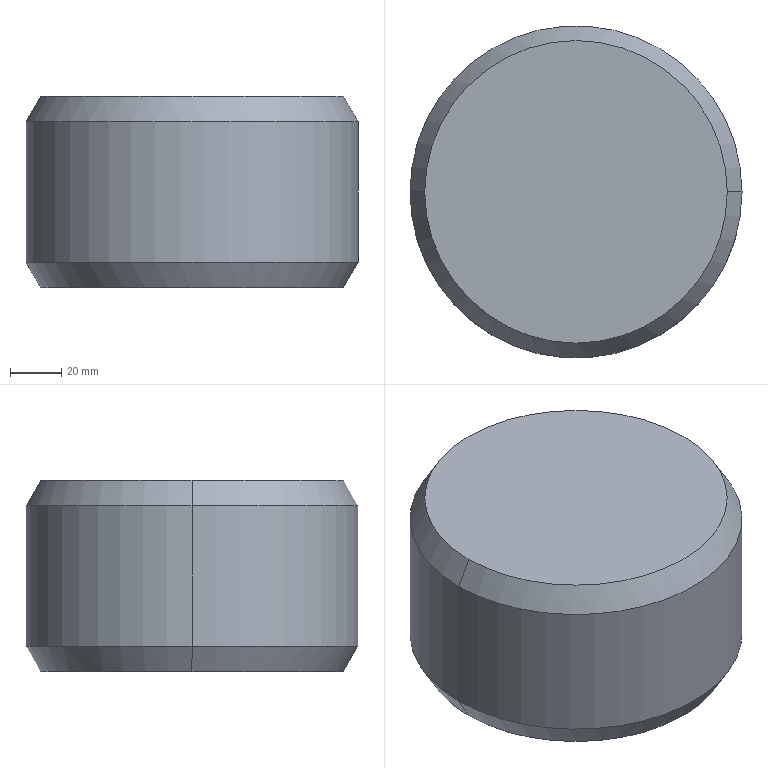Part | SolidWorks | features Chamfer 1, Extrusion 1 | 1 solid | 8 faces | box 130 x 130 x 75 mm | volume 972611 mm3 | cone 4 | cylinder 2 | plane 2 | commonest cylinder face diameters 130 x2
STEP:
#1=CARTESIAN_POINT('',(-59.226,0.,0.));
#2=VERTEX_POINT('',#1);
#3=CARTESIAN_POINT('',(59.226,0.,0.));
#4=VERTEX_POINT('',#3);
#5=CARTESIAN_POINT('',(0.,0.,0.));
#6=DIRECTION('',(0.,0.,-1.));
#7=DIRECTION('',(1.,0.,0.));
#8=AXIS2_PLACEMENT_3D('',#5,#6,#7);
#9=CIRCLE('',#8,59.226);
#10=EDGE_CURVE('',#2,#4,#9,.T.);
#11=ORIENTED_EDGE('',*,*,#10,.F.);
#12=CARTESIAN_POINT('',(-65.,0.,10.));
#13=VERTEX_POINT('',#12);
#14=CARTESIAN_POINT('',(-65.,0.,10.));
#15=DIRECTION('',(-0.5,0.,0.866));
#16=VECTOR('',#15,1000.);
#17=LINE('',#14,#16);
#18=EDGE_CURVE('',#2,#13,#17,.T.);
#19=ORIENTED_EDGE('',*,*,#18,.T.);
#20=CARTESIAN_POINT('',(65.,0.,10.));
#21=VERTEX_POINT('',#20);
#22=CARTESIAN_POINT('',(0.,0.,10.));
#23=DIRECTION('',(0.,0.,1.));
#24=DIRECTION('',(1.,0.,0.));
#25=AXIS2_PLACEMENT_3D('',#22,#23,#24);
#26=CIRCLE('',#25,65.);
#27=EDGE_CURVE('',#21,#13,#26,.T.);
#28=ORIENTED_EDGE('',*,*,#27,.F.);
#29=CARTESIAN_POINT('',(65.,0.,10.));
#30=DIRECTION('',(0.5,0.,0.866));
#31=VECTOR('',#30,1000.);
#32=LINE('',#29,#31);
#33=EDGE_CURVE('',#4,#21,#32,.T.);
#34=ORIENTED_EDGE('',*,*,#33,.F.);
#35=EDGE_LOOP('',(#11,#19,#28,#34));
#36=FACE_OUTER_BOUND('',#35,.T.);
#37=CARTESIAN_POINT('',(0.,0.,10.));
#38=DIRECTION('',(0.,0.,1.));
#39=DIRECTION('',(1.,0.,0.));
#40=AXIS2_PLACEMENT_3D('',#37,#38,#39);
#41=CONICAL_SURFACE('',#40,65.,0.5236);
#42=ADVANCED_FACE('',(#36),#41,.T.);
#43=CARTESIAN_POINT('',(59.226,0.,75.));
#44=VERTEX_POINT('',#43);
#45=CARTESIAN_POINT('',(-59.226,0.,75.));
#46=VERTEX_POINT('',#45);
#47=CARTESIAN_POINT('',(0.,0.,75.));
#48=DIRECTION('',(0.,0.,1.));
#49=DIRECTION('',(1.,0.,0.));
#50=AXIS2_PLACEMENT_3D('',#47,#48,#49);
#51=CIRCLE('',#50,59.226);
#52=EDGE_CURVE('',#44,#46,#51,.T.);
#53=ORIENTED_EDGE('',*,*,#52,.F.);
#54=CARTESIAN_POINT('',(65.,0.,65.));
#55=VERTEX_POINT('',#54);
#56=CARTESIAN_POINT('',(59.226,0.,75.));
#57=DIRECTION('',(0.5,0.,-0.866));
#58=VECTOR('',#57,1000.);
#59=LINE('',#56,#58);
#60=EDGE_CURVE('',#44,#55,#59,.T.);
#61=ORIENTED_EDGE('',*,*,#60,.T.);
#62=CARTESIAN_POINT('',(-65.,0.,65.));
#63=VERTEX_POINT('',#62);
#64=CARTESIAN_POINT('',(0.,0.,65.));
#65=DIRECTION('',(0.,0.,-1.));
#66=DIRECTION('',(1.,0.,0.));
#67=AXIS2_PLACEMENT_3D('',#64,#65,#66);
#68=CIRCLE('',#67,65.);
#69=EDGE_CURVE('',#63,#55,#68,.T.);
#70=ORIENTED_EDGE('',*,*,#69,.F.);
#71=CARTESIAN_POINT('',(-59.226,0.,75.));
#72=DIRECTION('',(-0.5,0.,-0.866));
#73=VECTOR('',#72,1000.);
#74=LINE('',#71,#73);
#75=EDGE_CURVE('',#46,#63,#74,.T.);
#76=ORIENTED_EDGE('',*,*,#75,.F.);
#77=EDGE_LOOP('',(#53,#61,#70,#76));
#78=FACE_OUTER_BOUND('',#77,.T.);
#79=CARTESIAN_POINT('',(0.,0.,75.));
#80=DIRECTION('',(0.,0.,-1.));
#81=DIRECTION('',(-1.,0.,0.));
#82=AXIS2_PLACEMENT_3D('',#79,#80,#81);
#83=CONICAL_SURFACE('',#82,59.226,0.5236);
#84=ADVANCED_FACE('',(#78),#83,.T.);
#85=ORIENTED_EDGE('',*,*,#69,.T.);
#86=CARTESIAN_POINT('',(65.,0.,75.));
#87=DIRECTION('',(0.,0.,-1.));
#88=VECTOR('',#87,1000.);
#89=LINE('',#86,#88);
#90=EDGE_CURVE('',#55,#21,#89,.T.);
#91=ORIENTED_EDGE('',*,*,#90,.T.);
#92=ORIENTED_EDGE('',*,*,#27,.T.);
#93=CARTESIAN_POINT('',(-65.,0.,75.));
#94=DIRECTION('',(0.,0.,-1.));
#95=VECTOR('',#94,1000.);
#96=LINE('',#93,#95);
#97=EDGE_CURVE('',#63,#13,#96,.T.);
#98=ORIENTED_EDGE('',*,*,#97,.F.);
#99=EDGE_LOOP('',(#85,#91,#92,#98));
#100=FACE_OUTER_BOUND('',#99,.T.);
#101=CARTESIAN_POINT('',(0.,0.,75.));
#102=DIRECTION('',(0.,0.,-1.));
#103=DIRECTION('',(-1.,0.,0.));
#104=AXIS2_PLACEMENT_3D('',#101,#102,#103);
#105=CYLINDRICAL_SURFACE('',#104,65.);
#106=ADVANCED_FACE('',(#100),#105,.T.);
#107=ORIENTED_EDGE('',*,*,#90,.F.);
#108=CARTESIAN_POINT('',(0.,0.,65.));
#109=DIRECTION('',(0.,0.,-1.));
#110=DIRECTION('',(1.,0.,0.));
#111=AXIS2_PLACEMENT_3D('',#108,#109,#110);
#112=CIRCLE('',#111,65.);
#113=EDGE_CURVE('',#55,#63,#112,.T.);
#114=ORIENTED_EDGE('',*,*,#113,.T.);
#115=ORIENTED_EDGE('',*,*,#97,.T.);
#116=CARTESIAN_POINT('',(0.,0.,10.));
#117=DIRECTION('',(0.,0.,1.));
#118=DIRECTION('',(1.,0.,0.));
#119=AXIS2_PLACEMENT_3D('',#116,#117,#118);
#120=CIRCLE('',#119,65.);
#121=EDGE_CURVE('',#13,#21,#120,.T.);
#122=ORIENTED_EDGE('',*,*,#121,.T.);
#123=EDGE_LOOP('',(#107,#114,#115,#122));
#124=FACE_OUTER_BOUND('',#123,.T.);
#125=CARTESIAN_POINT('',(0.,0.,75.));
#126=DIRECTION('',(0.,0.,-1.));
#127=DIRECTION('',(-1.,0.,0.));
#128=AXIS2_PLACEMENT_3D('',#125,#126,#127);
#129=CYLINDRICAL_SURFACE('',#128,65.);
#130=ADVANCED_FACE('',(#124),#129,.T.);
#131=CARTESIAN_POINT('',(0.,0.,75.));
#132=DIRECTION('',(0.,0.,1.));
#133=DIRECTION('',(1.,0.,0.));
#134=AXIS2_PLACEMENT_3D('',#131,#132,#133);
#135=CIRCLE('',#134,59.226);
#136=EDGE_CURVE('',#46,#44,#135,.T.);
#137=ORIENTED_EDGE('',*,*,#136,.T.);
#138=ORIENTED_EDGE('',*,*,#52,.T.);
#139=EDGE_LOOP('',(#137,#138));
#140=FACE_OUTER_BOUND('',#139,.T.);
#141=CARTESIAN_POINT('',(0.,0.,75.));
#142=DIRECTION('',(0.,0.,1.));
#143=DIRECTION('',(1.,0.,0.));
#144=AXIS2_PLACEMENT_3D('',#141,#142,#143);
#145=PLANE('',#144);
#146=ADVANCED_FACE('',(#140),#145,.T.);
#147=CARTESIAN_POINT('',(0.,0.,0.));
#148=DIRECTION('',(0.,0.,-1.));
#149=DIRECTION('',(1.,0.,0.));
#150=AXIS2_PLACEMENT_3D('',#147,#148,#149);
#151=CIRCLE('',#150,59.226);
#152=EDGE_CURVE('',#4,#2,#151,.T.);
#153=ORIENTED_EDGE('',*,*,#152,.T.);
#154=ORIENTED_EDGE('',*,*,#10,.T.);
#155=EDGE_LOOP('',(#153,#154));
#156=FACE_OUTER_BOUND('',#155,.T.);
#157=CARTESIAN_POINT('',(0.,0.,0.));
#158=DIRECTION('',(0.,0.,1.));
#159=DIRECTION('',(1.,0.,0.));
#160=AXIS2_PLACEMENT_3D('',#157,#158,#159);
#161=PLANE('',#160);
#162=ADVANCED_FACE('',(#156),#161,.F.);
#163=ORIENTED_EDGE('',*,*,#60,.F.);
#164=ORIENTED_EDGE('',*,*,#136,.F.);
#165=ORIENTED_EDGE('',*,*,#75,.T.);
#166=ORIENTED_EDGE('',*,*,#113,.F.);
#167=EDGE_LOOP('',(#163,#164,#165,#166));
#168=FACE_OUTER_BOUND('',#167,.T.);
#169=CARTESIAN_POINT('',(0.,0.,75.));
#170=DIRECTION('',(0.,0.,-1.));
#171=DIRECTION('',(-1.,0.,0.));
#172=AXIS2_PLACEMENT_3D('',#169,#170,#171);
#173=CONICAL_SURFACE('',#172,59.226,0.5236);
#174=ADVANCED_FACE('',(#168),#173,.T.);
#175=ORIENTED_EDGE('',*,*,#18,.F.);
#176=ORIENTED_EDGE('',*,*,#152,.F.);
#177=ORIENTED_EDGE('',*,*,#33,.T.);
#178=ORIENTED_EDGE('',*,*,#121,.F.);
#179=EDGE_LOOP('',(#175,#176,#177,#178));
#180=FACE_OUTER_BOUND('',#179,.T.);
#181=CARTESIAN_POINT('',(0.,0.,10.));
#182=DIRECTION('',(0.,0.,1.));
#183=DIRECTION('',(1.,0.,0.));
#184=AXIS2_PLACEMENT_3D('',#181,#182,#183);
#185=CONICAL_SURFACE('',#184,65.,0.5236);
#186=ADVANCED_FACE('',(#180),#185,.T.);
#187=CLOSED_SHELL('',(#42,#84,#106,#130,#146,#162,#174,#186));
#188=MANIFOLD_SOLID_BREP('',#187);
#189=CARTESIAN_POINT('',(0.,0.,0.));
#190=DIRECTION('',(0.,0.,1.));
#191=DIRECTION('',(1.,0.,0.));
#192=AXIS2_PLACEMENT_3D('',#189,#190,#191);
#193=(LENGTH_UNIT()NAMED_UNIT(*)SI_UNIT(.MILLI.,.METRE.));
#194=UNCERTAINTY_MEASURE_WITH_UNIT(LENGTH_MEASURE(0.00001),#193,'','');
#195=(NAMED_UNIT(*)PLANE_ANGLE_UNIT()SI_UNIT($,.RADIAN.));
#196=(NAMED_UNIT(*)SI_UNIT($,.STERADIAN.)SOLID_ANGLE_UNIT());
#197=(GEOMETRIC_REPRESENTATION_CONTEXT(3)GLOBAL_UNCERTAINTY_ASSIGNED_CONTEXT((#194))GLOBAL_UNIT_ASSIGNED_CONTEXT((#193,#195,#196))REPRESENTATION_CONTEXT('',''));
#198=ADVANCED_BREP_SHAPE_REPRESENTATION('',(#188,#192),#197);